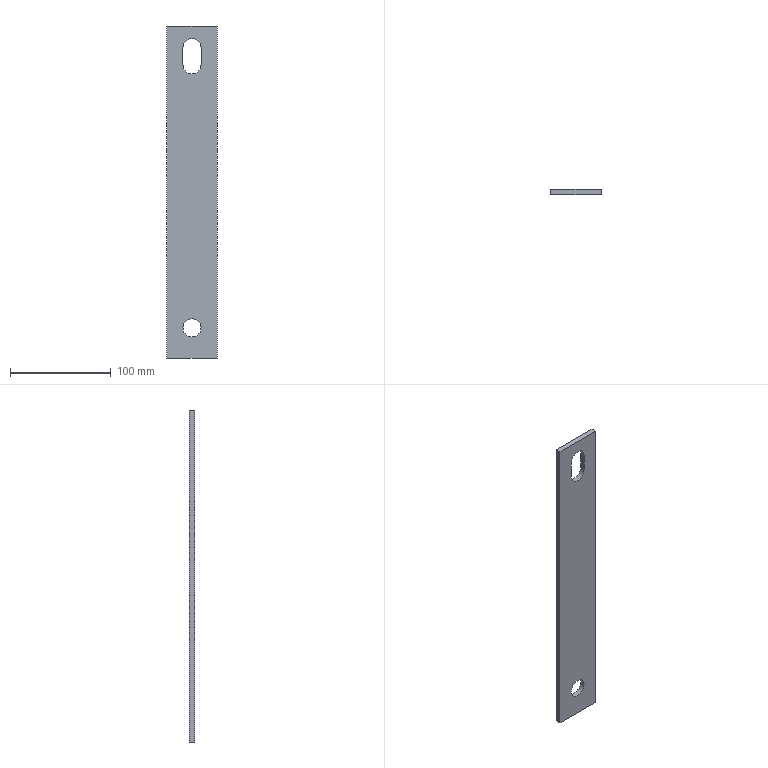Part | NX | features solid 2 | 1 solid | 11 faces | box 50 x 5 x 330 mm | volume 78425 mm3 | plane 8 | cylinder 3 | commonest cylinder face diameters 18 x3
STEP:
#1=CARTESIAN_POINT('',(855.,-415.,-175.));
#2=VERTEX_POINT('',#1);
#3=CARTESIAN_POINT('',(805.,-415.,-175.));
#4=VERTEX_POINT('',#3);
#5=CARTESIAN_POINT('',(855.,-415.,-175.));
#6=DIRECTION('',(-1.,0.,0.));
#7=VECTOR('',#6,1000.);
#8=LINE('',#5,#7);
#9=EDGE_CURVE('',#2,#4,#8,.T.);
#10=ORIENTED_EDGE('',*,*,#9,.F.);
#11=CARTESIAN_POINT('',(855.,-420.,-175.));
#12=VERTEX_POINT('',#11);
#13=CARTESIAN_POINT('',(855.,-420.,-175.));
#14=DIRECTION('',(0.,1.,0.));
#15=VECTOR('',#14,1000.);
#16=LINE('',#13,#15);
#17=EDGE_CURVE('',#12,#2,#16,.T.);
#18=ORIENTED_EDGE('',*,*,#17,.F.);
#19=CARTESIAN_POINT('',(805.,-420.,-175.));
#20=VERTEX_POINT('',#19);
#21=CARTESIAN_POINT('',(855.,-420.,-175.));
#22=DIRECTION('',(-1.,0.,0.));
#23=VECTOR('',#22,1000.);
#24=LINE('',#21,#23);
#25=EDGE_CURVE('',#12,#20,#24,.T.);
#26=ORIENTED_EDGE('',*,*,#25,.T.);
#27=CARTESIAN_POINT('',(805.,-420.,-175.));
#28=DIRECTION('',(0.,1.,0.));
#29=VECTOR('',#28,1000.);
#30=LINE('',#27,#29);
#31=EDGE_CURVE('',#20,#4,#30,.T.);
#32=ORIENTED_EDGE('',*,*,#31,.T.);
#33=EDGE_LOOP('',(#10,#18,#26,#32));
#34=FACE_BOUND('',#33,.T.);
#35=CARTESIAN_POINT('',(855.,-420.,-175.));
#36=DIRECTION('',(0.,0.,-1.));
#37=DIRECTION('',(0.,-1.,0.));
#38=AXIS2_PLACEMENT_3D('',#35,#36,#37);
#39=PLANE('',#38);
#40=ADVANCED_FACE('',(#34),#39,.T.);
#41=CARTESIAN_POINT('',(821.,-420.,-145.));
#42=VERTEX_POINT('',#41);
#43=CARTESIAN_POINT('',(830.,-420.,-145.));
#44=DIRECTION('',(0.,1.,0.));
#45=DIRECTION('',(-1.,0.,0.));
#46=AXIS2_PLACEMENT_3D('',#43,#44,#45);
#47=CIRCLE('',#46,9.);
#48=EDGE_CURVE('',#42,#42,#47,.T.);
#49=ORIENTED_EDGE('',*,*,#48,.F.);
#50=EDGE_LOOP('',(#49));
#51=FACE_BOUND('',#50,.T.);
#52=CARTESIAN_POINT('',(821.,-415.,-145.));
#53=VERTEX_POINT('',#52);
#54=CARTESIAN_POINT('',(830.,-415.,-145.));
#55=DIRECTION('',(0.,1.,0.));
#56=DIRECTION('',(-1.,0.,0.));
#57=AXIS2_PLACEMENT_3D('',#54,#55,#56);
#58=CIRCLE('',#57,9.);
#59=EDGE_CURVE('',#53,#53,#58,.T.);
#60=ORIENTED_EDGE('',*,*,#59,.T.);
#61=EDGE_LOOP('',(#60));
#62=FACE_BOUND('',#61,.T.);
#63=CARTESIAN_POINT('',(830.,-420.,-145.));
#64=DIRECTION('',(0.,1.,0.));
#65=DIRECTION('',(-1.,0.,0.));
#66=AXIS2_PLACEMENT_3D('',#63,#64,#65);
#67=CYLINDRICAL_SURFACE('',#66,9.);
#68=ADVANCED_FACE('',(#51,#62),#67,.F.);
#69=ORIENTED_EDGE('',*,*,#48,.T.);
#70=EDGE_LOOP('',(#69));
#71=FACE_BOUND('',#70,.T.);
#72=CARTESIAN_POINT('',(855.,-420.,155.));
#73=VERTEX_POINT('',#72);
#74=CARTESIAN_POINT('',(855.,-420.,105.));
#75=DIRECTION('',(0.,0.,-1.));
#76=VECTOR('',#75,1000.);
#77=LINE('',#74,#76);
#78=EDGE_CURVE('',#73,#12,#77,.T.);
#79=ORIENTED_EDGE('',*,*,#78,.F.);
#80=CARTESIAN_POINT('',(805.,-420.,155.));
#81=VERTEX_POINT('',#80);
#82=CARTESIAN_POINT('',(805.,-420.,155.));
#83=DIRECTION('',(1.,0.,0.));
#84=VECTOR('',#83,1000.);
#85=LINE('',#82,#84);
#86=EDGE_CURVE('',#81,#73,#85,.T.);
#87=ORIENTED_EDGE('',*,*,#86,.F.);
#88=CARTESIAN_POINT('',(805.,-420.,-175.));
#89=DIRECTION('',(0.,0.,1.));
#90=VECTOR('',#89,1000.);
#91=LINE('',#88,#90);
#92=EDGE_CURVE('',#20,#81,#91,.T.);
#93=ORIENTED_EDGE('',*,*,#92,.F.);
#94=ORIENTED_EDGE('',*,*,#25,.F.);
#95=EDGE_LOOP('',(#79,#87,#93,#94));
#96=FACE_BOUND('',#95,.T.);
#97=CARTESIAN_POINT('',(821.,-420.,133.5));
#98=VERTEX_POINT('',#97);
#99=CARTESIAN_POINT('',(839.,-420.,133.5));
#100=VERTEX_POINT('',#99);
#101=CARTESIAN_POINT('',(830.,-420.,133.5));
#102=DIRECTION('',(0.,1.,0.));
#103=DIRECTION('',(-1.,0.,0.));
#104=AXIS2_PLACEMENT_3D('',#101,#102,#103);
#105=CIRCLE('',#104,9.);
#106=EDGE_CURVE('',#98,#100,#105,.T.);
#107=ORIENTED_EDGE('',*,*,#106,.T.);
#108=CARTESIAN_POINT('',(839.,-420.,116.5));
#109=VERTEX_POINT('',#108);
#110=CARTESIAN_POINT('',(839.,-420.,116.5));
#111=DIRECTION('',(0.,0.,1.));
#112=VECTOR('',#111,1000.);
#113=LINE('',#110,#112);
#114=EDGE_CURVE('',#109,#100,#113,.T.);
#115=ORIENTED_EDGE('',*,*,#114,.F.);
#116=CARTESIAN_POINT('',(821.,-420.,116.5));
#117=VERTEX_POINT('',#116);
#118=CARTESIAN_POINT('',(830.,-420.,116.5));
#119=DIRECTION('',(0.,1.,0.));
#120=DIRECTION('',(-1.,0.,0.));
#121=AXIS2_PLACEMENT_3D('',#118,#119,#120);
#122=CIRCLE('',#121,9.);
#123=EDGE_CURVE('',#109,#117,#122,.T.);
#124=ORIENTED_EDGE('',*,*,#123,.T.);
#125=CARTESIAN_POINT('',(821.,-420.,133.5));
#126=DIRECTION('',(0.,0.,-1.));
#127=VECTOR('',#126,1000.);
#128=LINE('',#125,#127);
#129=EDGE_CURVE('',#98,#117,#128,.T.);
#130=ORIENTED_EDGE('',*,*,#129,.F.);
#131=EDGE_LOOP('',(#107,#115,#124,#130));
#132=FACE_BOUND('',#131,.T.);
#133=CARTESIAN_POINT('',(805.,-420.,105.));
#134=DIRECTION('',(0.,1.,0.));
#135=DIRECTION('',(-1.,0.,0.));
#136=AXIS2_PLACEMENT_3D('',#133,#134,#135);
#137=PLANE('',#136);
#138=ADVANCED_FACE('',(#71,#96,#132),#137,.F.);
#139=ORIENTED_EDGE('',*,*,#59,.F.);
#140=EDGE_LOOP('',(#139));
#141=FACE_BOUND('',#140,.T.);
#142=CARTESIAN_POINT('',(805.,-415.,155.));
#143=VERTEX_POINT('',#142);
#144=CARTESIAN_POINT('',(805.,-415.,-175.));
#145=DIRECTION('',(0.,0.,1.));
#146=VECTOR('',#145,1000.);
#147=LINE('',#144,#146);
#148=EDGE_CURVE('',#4,#143,#147,.T.);
#149=ORIENTED_EDGE('',*,*,#148,.T.);
#150=CARTESIAN_POINT('',(855.,-415.,155.));
#151=VERTEX_POINT('',#150);
#152=CARTESIAN_POINT('',(805.,-415.,155.));
#153=DIRECTION('',(1.,0.,0.));
#154=VECTOR('',#153,1000.);
#155=LINE('',#152,#154);
#156=EDGE_CURVE('',#143,#151,#155,.T.);
#157=ORIENTED_EDGE('',*,*,#156,.T.);
#158=CARTESIAN_POINT('',(855.,-415.,105.));
#159=DIRECTION('',(0.,0.,-1.));
#160=VECTOR('',#159,1000.);
#161=LINE('',#158,#160);
#162=EDGE_CURVE('',#151,#2,#161,.T.);
#163=ORIENTED_EDGE('',*,*,#162,.T.);
#164=ORIENTED_EDGE('',*,*,#9,.T.);
#165=EDGE_LOOP('',(#149,#157,#163,#164));
#166=FACE_BOUND('',#165,.T.);
#167=CARTESIAN_POINT('',(821.,-415.,133.5));
#168=VERTEX_POINT('',#167);
#169=CARTESIAN_POINT('',(839.,-415.,133.5));
#170=VERTEX_POINT('',#169);
#171=CARTESIAN_POINT('',(830.,-415.,133.5));
#172=DIRECTION('',(0.,1.,0.));
#173=DIRECTION('',(-1.,0.,0.));
#174=AXIS2_PLACEMENT_3D('',#171,#172,#173);
#175=CIRCLE('',#174,9.);
#176=EDGE_CURVE('',#168,#170,#175,.T.);
#177=ORIENTED_EDGE('',*,*,#176,.F.);
#178=CARTESIAN_POINT('',(821.,-415.,116.5));
#179=VERTEX_POINT('',#178);
#180=CARTESIAN_POINT('',(821.,-415.,133.5));
#181=DIRECTION('',(0.,0.,-1.));
#182=VECTOR('',#181,1000.);
#183=LINE('',#180,#182);
#184=EDGE_CURVE('',#168,#179,#183,.T.);
#185=ORIENTED_EDGE('',*,*,#184,.T.);
#186=CARTESIAN_POINT('',(839.,-415.,116.5));
#187=VERTEX_POINT('',#186);
#188=CARTESIAN_POINT('',(830.,-415.,116.5));
#189=DIRECTION('',(0.,1.,0.));
#190=DIRECTION('',(-1.,0.,0.));
#191=AXIS2_PLACEMENT_3D('',#188,#189,#190);
#192=CIRCLE('',#191,9.);
#193=EDGE_CURVE('',#187,#179,#192,.T.);
#194=ORIENTED_EDGE('',*,*,#193,.F.);
#195=CARTESIAN_POINT('',(839.,-415.,116.5));
#196=DIRECTION('',(0.,0.,1.));
#197=VECTOR('',#196,1000.);
#198=LINE('',#195,#197);
#199=EDGE_CURVE('',#187,#170,#198,.T.);
#200=ORIENTED_EDGE('',*,*,#199,.T.);
#201=EDGE_LOOP('',(#177,#185,#194,#200));
#202=FACE_BOUND('',#201,.T.);
#203=CARTESIAN_POINT('',(805.,-415.,105.));
#204=DIRECTION('',(0.,1.,0.));
#205=DIRECTION('',(-1.,0.,0.));
#206=AXIS2_PLACEMENT_3D('',#203,#204,#205);
#207=PLANE('',#206);
#208=ADVANCED_FACE('',(#141,#166,#202),#207,.T.);
#209=ORIENTED_EDGE('',*,*,#162,.F.);
#210=CARTESIAN_POINT('',(855.,-420.,155.));
#211=DIRECTION('',(0.,1.,0.));
#212=VECTOR('',#211,1000.);
#213=LINE('',#210,#212);
#214=EDGE_CURVE('',#73,#151,#213,.T.);
#215=ORIENTED_EDGE('',*,*,#214,.F.);
#216=ORIENTED_EDGE('',*,*,#78,.T.);
#217=ORIENTED_EDGE('',*,*,#17,.T.);
#218=EDGE_LOOP('',(#209,#215,#216,#217));
#219=FACE_BOUND('',#218,.T.);
#220=CARTESIAN_POINT('',(855.,-420.,105.));
#221=DIRECTION('',(1.,0.,0.));
#222=DIRECTION('',(0.,0.,-1.));
#223=AXIS2_PLACEMENT_3D('',#220,#221,#222);
#224=PLANE('',#223);
#225=ADVANCED_FACE('',(#219),#224,.T.);
#226=ORIENTED_EDGE('',*,*,#92,.T.);
#227=CARTESIAN_POINT('',(805.,-420.,155.));
#228=DIRECTION('',(0.,1.,0.));
#229=VECTOR('',#228,1000.);
#230=LINE('',#227,#229);
#231=EDGE_CURVE('',#81,#143,#230,.T.);
#232=ORIENTED_EDGE('',*,*,#231,.T.);
#233=ORIENTED_EDGE('',*,*,#148,.F.);
#234=ORIENTED_EDGE('',*,*,#31,.F.);
#235=EDGE_LOOP('',(#226,#232,#233,#234));
#236=FACE_BOUND('',#235,.T.);
#237=CARTESIAN_POINT('',(805.,-420.,-175.));
#238=DIRECTION('',(-1.,0.,0.));
#239=DIRECTION('',(0.,0.,1.));
#240=AXIS2_PLACEMENT_3D('',#237,#238,#239);
#241=PLANE('',#240);
#242=ADVANCED_FACE('',(#236),#241,.T.);
#243=ORIENTED_EDGE('',*,*,#176,.T.);
#244=CARTESIAN_POINT('',(839.,-420.,133.5));
#245=DIRECTION('',(0.,1.,0.));
#246=VECTOR('',#245,1000.);
#247=LINE('',#244,#246);
#248=EDGE_CURVE('',#100,#170,#247,.T.);
#249=ORIENTED_EDGE('',*,*,#248,.F.);
#250=ORIENTED_EDGE('',*,*,#106,.F.);
#251=CARTESIAN_POINT('',(821.,-420.,133.5));
#252=DIRECTION('',(0.,1.,0.));
#253=VECTOR('',#252,1000.);
#254=LINE('',#251,#253);
#255=EDGE_CURVE('',#98,#168,#254,.T.);
#256=ORIENTED_EDGE('',*,*,#255,.T.);
#257=EDGE_LOOP('',(#243,#249,#250,#256));
#258=FACE_BOUND('',#257,.T.);
#259=CARTESIAN_POINT('',(830.,-420.,133.5));
#260=DIRECTION('',(0.,1.,0.));
#261=DIRECTION('',(-1.,0.,0.));
#262=AXIS2_PLACEMENT_3D('',#259,#260,#261);
#263=CYLINDRICAL_SURFACE('',#262,9.);
#264=ADVANCED_FACE('',(#258),#263,.F.);
#265=ORIENTED_EDGE('',*,*,#184,.F.);
#266=ORIENTED_EDGE('',*,*,#255,.F.);
#267=ORIENTED_EDGE('',*,*,#129,.T.);
#268=CARTESIAN_POINT('',(821.,-420.,116.5));
#269=DIRECTION('',(0.,1.,0.));
#270=VECTOR('',#269,1000.);
#271=LINE('',#268,#270);
#272=EDGE_CURVE('',#117,#179,#271,.T.);
#273=ORIENTED_EDGE('',*,*,#272,.T.);
#274=EDGE_LOOP('',(#265,#266,#267,#273));
#275=FACE_BOUND('',#274,.T.);
#276=CARTESIAN_POINT('',(821.,-420.,133.5));
#277=DIRECTION('',(1.,0.,0.));
#278=DIRECTION('',(0.,1.,0.));
#279=AXIS2_PLACEMENT_3D('',#276,#277,#278);
#280=PLANE('',#279);
#281=ADVANCED_FACE('',(#275),#280,.T.);
#282=ORIENTED_EDGE('',*,*,#193,.T.);
#283=ORIENTED_EDGE('',*,*,#272,.F.);
#284=ORIENTED_EDGE('',*,*,#123,.F.);
#285=CARTESIAN_POINT('',(839.,-420.,116.5));
#286=DIRECTION('',(0.,1.,0.));
#287=VECTOR('',#286,1000.);
#288=LINE('',#285,#287);
#289=EDGE_CURVE('',#109,#187,#288,.T.);
#290=ORIENTED_EDGE('',*,*,#289,.T.);
#291=EDGE_LOOP('',(#282,#283,#284,#290));
#292=FACE_BOUND('',#291,.T.);
#293=CARTESIAN_POINT('',(830.,-420.,116.5));
#294=DIRECTION('',(0.,1.,0.));
#295=DIRECTION('',(-1.,0.,0.));
#296=AXIS2_PLACEMENT_3D('',#293,#294,#295);
#297=CYLINDRICAL_SURFACE('',#296,9.);
#298=ADVANCED_FACE('',(#292),#297,.F.);
#299=ORIENTED_EDGE('',*,*,#156,.F.);
#300=ORIENTED_EDGE('',*,*,#231,.F.);
#301=ORIENTED_EDGE('',*,*,#86,.T.);
#302=ORIENTED_EDGE('',*,*,#214,.T.);
#303=EDGE_LOOP('',(#299,#300,#301,#302));
#304=FACE_BOUND('',#303,.T.);
#305=CARTESIAN_POINT('',(805.,-420.,155.));
#306=DIRECTION('',(0.,0.,1.));
#307=DIRECTION('',(0.,1.,0.));
#308=AXIS2_PLACEMENT_3D('',#305,#306,#307);
#309=PLANE('',#308);
#310=ADVANCED_FACE('',(#304),#309,.T.);
#311=ORIENTED_EDGE('',*,*,#199,.F.);
#312=ORIENTED_EDGE('',*,*,#289,.F.);
#313=ORIENTED_EDGE('',*,*,#114,.T.);
#314=ORIENTED_EDGE('',*,*,#248,.T.);
#315=EDGE_LOOP('',(#311,#312,#313,#314));
#316=FACE_BOUND('',#315,.T.);
#317=CARTESIAN_POINT('',(839.,-420.,116.5));
#318=DIRECTION('',(-1.,0.,0.));
#319=DIRECTION('',(0.,-1.,0.));
#320=AXIS2_PLACEMENT_3D('',#317,#318,#319);
#321=PLANE('',#320);
#322=ADVANCED_FACE('',(#316),#321,.T.);
#323=CLOSED_SHELL('',(#40,#68,#138,#208,#225,#242,#264,#281,#298,#310,#322));
#324=MANIFOLD_SOLID_BREP('',#323);
#325=(LENGTH_UNIT()NAMED_UNIT(*)SI_UNIT(.MILLI.,.METRE.));
#326=UNCERTAINTY_MEASURE_WITH_UNIT(LENGTH_MEASURE(0.00001),#325,'','');
#327=(NAMED_UNIT(*)PLANE_ANGLE_UNIT()SI_UNIT($,.RADIAN.));
#328=(NAMED_UNIT(*)SI_UNIT($,.STERADIAN.)SOLID_ANGLE_UNIT());
#329=(GEOMETRIC_REPRESENTATION_CONTEXT(3)GLOBAL_UNCERTAINTY_ASSIGNED_CONTEXT((#326))GLOBAL_UNIT_ASSIGNED_CONTEXT((#325,#327,#328))REPRESENTATION_CONTEXT('',''));
#330=ADVANCED_BREP_SHAPE_REPRESENTATION('',(#324),#329);